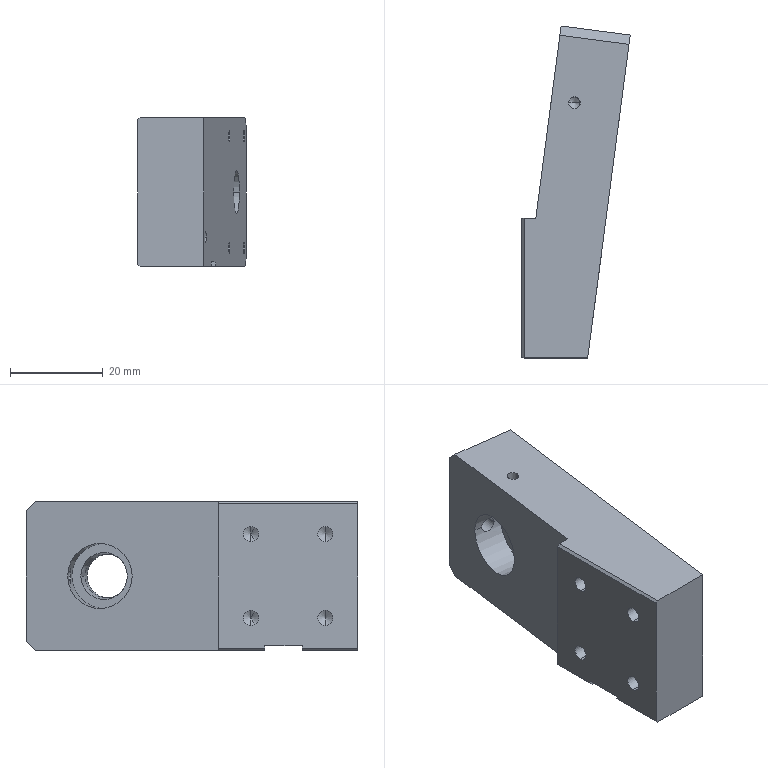Part | SolidWorks | features HoleWzd 7, Chamfer 3, ICE 3, Extrusion 1, MirrorPattern 1, RevCut 1 | 1 solid | 90 faces | box 23.317 x 71.359 x 32 mm | volume 32311 mm3 | cylinder 40 | cone 32 | plane 18 | commonest cylinder face diameters 2.5 x22 3.3 x10 1.2 x4 9.5 x2 14 x2